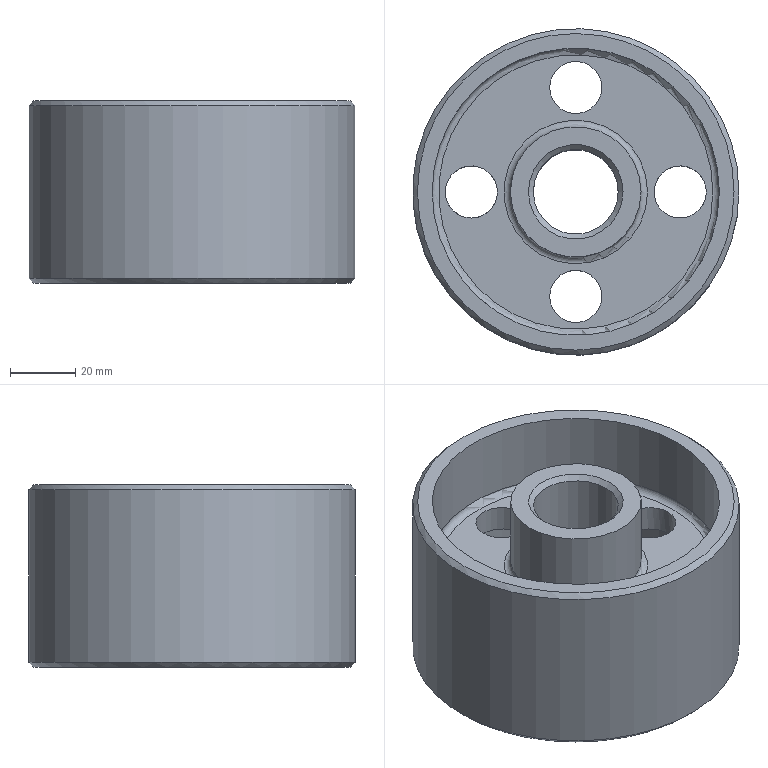Part | NX | features EXTRUDE 5, DATUM_CSYS 3, CHAMFER 2, SKETCH 2, BLEND 1 | 1 solid | 24 faces | box 100 x 100 x 56 mm | volume 171833 mm3 | cylinder 10 | plane 6 | cone 4 | torus 4 | commonest cylinder face diameters 16 x4 40 x2 88 x2 26 x1 100 x1
STEP:
#1=CARTESIAN_POINT('',(14.5,0.,56.));
#2=VERTEX_POINT('',#1);
#3=CARTESIAN_POINT('',(0.,0.,56.));
#4=DIRECTION('',(0.,0.,1.));
#5=DIRECTION('',(1.,0.,0.));
#6=AXIS2_PLACEMENT_3D('',#3,#4,#5);
#7=CIRCLE('',#6,14.5);
#8=EDGE_CURVE('',#2,#2,#7,.F.);
#9=ORIENTED_EDGE('',*,*,#8,.T.);
#10=EDGE_LOOP('',(#9));
#11=FACE_BOUND('',#10,.T.);
#12=CARTESIAN_POINT('',(20.,0.,56.));
#13=VERTEX_POINT('',#12);
#14=CARTESIAN_POINT('',(0.,0.,56.));
#15=DIRECTION('',(0.,0.,1.));
#16=DIRECTION('',(1.,0.,0.));
#17=AXIS2_PLACEMENT_3D('',#14,#15,#16);
#18=CIRCLE('',#17,20.);
#19=EDGE_CURVE('',#13,#13,#18,.T.);
#20=ORIENTED_EDGE('',*,*,#19,.T.);
#21=EDGE_LOOP('',(#20));
#22=FACE_BOUND('',#21,.T.);
#23=CARTESIAN_POINT('',(0.,0.,56.));
#24=DIRECTION('',(0.,0.,1.));
#25=DIRECTION('',(1.,0.,0.));
#26=AXIS2_PLACEMENT_3D('',#23,#24,#25);
#27=PLANE('',#26);
#28=ADVANCED_FACE('',(#11,#22),#27,.T.);
#29=CARTESIAN_POINT('',(48.5,0.,0.));
#30=VERTEX_POINT('',#29);
#31=CARTESIAN_POINT('',(0.,0.,0.));
#32=DIRECTION('',(0.,0.,1.));
#33=DIRECTION('',(1.,0.,0.));
#34=AXIS2_PLACEMENT_3D('',#31,#32,#33);
#35=CIRCLE('',#34,48.5);
#36=EDGE_CURVE('',#30,#30,#35,.F.);
#37=ORIENTED_EDGE('',*,*,#36,.T.);
#38=EDGE_LOOP('',(#37));
#39=FACE_BOUND('',#38,.T.);
#40=CARTESIAN_POINT('',(44.,0.,0.));
#41=VERTEX_POINT('',#40);
#42=CARTESIAN_POINT('',(0.,0.,0.));
#43=DIRECTION('',(0.,0.,-1.));
#44=DIRECTION('',(1.,0.,0.));
#45=AXIS2_PLACEMENT_3D('',#42,#43,#44);
#46=CIRCLE('',#45,44.);
#47=EDGE_CURVE('',#41,#41,#46,.T.);
#48=ORIENTED_EDGE('',*,*,#47,.F.);
#49=EDGE_LOOP('',(#48));
#50=FACE_BOUND('',#49,.T.);
#51=CARTESIAN_POINT('',(0.,0.,0.));
#52=DIRECTION('',(0.,0.,1.));
#53=DIRECTION('',(1.,0.,0.));
#54=AXIS2_PLACEMENT_3D('',#51,#52,#53);
#55=PLANE('',#54);
#56=ADVANCED_FACE('',(#39,#50),#55,.F.);
#57=CARTESIAN_POINT('',(14.5,0.,0.));
#58=VERTEX_POINT('',#57);
#59=CARTESIAN_POINT('',(0.,0.,0.));
#60=DIRECTION('',(0.,0.,1.));
#61=DIRECTION('',(1.,0.,0.));
#62=AXIS2_PLACEMENT_3D('',#59,#60,#61);
#63=CIRCLE('',#62,14.5);
#64=EDGE_CURVE('',#58,#58,#63,.T.);
#65=ORIENTED_EDGE('',*,*,#64,.T.);
#66=EDGE_LOOP('',(#65));
#67=FACE_BOUND('',#66,.T.);
#68=CARTESIAN_POINT('',(20.,0.,0.));
#69=VERTEX_POINT('',#68);
#70=CARTESIAN_POINT('',(0.,0.,0.));
#71=DIRECTION('',(0.,0.,1.));
#72=DIRECTION('',(1.,0.,0.));
#73=AXIS2_PLACEMENT_3D('',#70,#71,#72);
#74=CIRCLE('',#73,20.);
#75=EDGE_CURVE('',#69,#69,#74,.T.);
#76=ORIENTED_EDGE('',*,*,#75,.F.);
#77=EDGE_LOOP('',(#76));
#78=FACE_BOUND('',#77,.T.);
#79=CARTESIAN_POINT('',(0.,0.,0.));
#80=DIRECTION('',(0.,0.,1.));
#81=DIRECTION('',(1.,0.,0.));
#82=AXIS2_PLACEMENT_3D('',#79,#80,#81);
#83=PLANE('',#82);
#84=ADVANCED_FACE('',(#67,#78),#83,.F.);
#85=CARTESIAN_POINT('',(50.,0.,1.5));
#86=VERTEX_POINT('',#85);
#87=CARTESIAN_POINT('',(0.,0.,1.5));
#88=DIRECTION('',(0.,0.,1.));
#89=DIRECTION('',(1.,0.,0.));
#90=AXIS2_PLACEMENT_3D('',#87,#88,#89);
#91=CIRCLE('',#90,50.);
#92=EDGE_CURVE('',#86,#86,#91,.T.);
#93=ORIENTED_EDGE('',*,*,#92,.T.);
#94=EDGE_LOOP('',(#93));
#95=FACE_BOUND('',#94,.T.);
#96=CARTESIAN_POINT('',(50.,0.,54.5));
#97=VERTEX_POINT('',#96);
#98=CARTESIAN_POINT('',(0.,0.,54.5));
#99=DIRECTION('',(0.,0.,1.));
#100=DIRECTION('',(1.,0.,0.));
#101=AXIS2_PLACEMENT_3D('',#98,#99,#100);
#102=CIRCLE('',#101,50.);
#103=EDGE_CURVE('',#97,#97,#102,.F.);
#104=ORIENTED_EDGE('',*,*,#103,.T.);
#105=EDGE_LOOP('',(#104));
#106=FACE_BOUND('',#105,.T.);
#107=CARTESIAN_POINT('',(0.,0.,56.));
#108=DIRECTION('',(0.,0.,-1.));
#109=DIRECTION('',(-1.,0.,0.));
#110=AXIS2_PLACEMENT_3D('',#107,#108,#109);
#111=CYLINDRICAL_SURFACE('',#110,50.);
#112=ADVANCED_FACE('',(#95,#106),#111,.T.);
#113=CARTESIAN_POINT('',(48.5,0.,56.));
#114=VERTEX_POINT('',#113);
#115=CARTESIAN_POINT('',(0.,0.,56.));
#116=DIRECTION('',(0.,0.,1.));
#117=DIRECTION('',(1.,0.,0.));
#118=AXIS2_PLACEMENT_3D('',#115,#116,#117);
#119=CIRCLE('',#118,48.5);
#120=EDGE_CURVE('',#114,#114,#119,.T.);
#121=ORIENTED_EDGE('',*,*,#120,.T.);
#122=EDGE_LOOP('',(#121));
#123=FACE_BOUND('',#122,.T.);
#124=CARTESIAN_POINT('',(44.,0.,56.));
#125=VERTEX_POINT('',#124);
#126=CARTESIAN_POINT('',(0.,0.,56.));
#127=DIRECTION('',(0.,0.,1.));
#128=DIRECTION('',(1.,0.,0.));
#129=AXIS2_PLACEMENT_3D('',#126,#127,#128);
#130=CIRCLE('',#129,44.);
#131=EDGE_CURVE('',#125,#125,#130,.T.);
#132=ORIENTED_EDGE('',*,*,#131,.F.);
#133=EDGE_LOOP('',(#132));
#134=FACE_BOUND('',#133,.T.);
#135=CARTESIAN_POINT('',(0.,0.,56.));
#136=DIRECTION('',(0.,0.,1.));
#137=DIRECTION('',(1.,0.,0.));
#138=AXIS2_PLACEMENT_3D('',#135,#136,#137);
#139=PLANE('',#138);
#140=ADVANCED_FACE('',(#123,#134),#139,.T.);
#141=CARTESIAN_POINT('',(13.,0.,54.5));
#142=VERTEX_POINT('',#141);
#143=CARTESIAN_POINT('',(0.,0.,54.5));
#144=DIRECTION('',(0.,0.,1.));
#145=DIRECTION('',(1.,0.,0.));
#146=AXIS2_PLACEMENT_3D('',#143,#144,#145);
#147=CIRCLE('',#146,13.);
#148=EDGE_CURVE('',#142,#142,#147,.T.);
#149=ORIENTED_EDGE('',*,*,#148,.T.);
#150=EDGE_LOOP('',(#149));
#151=FACE_BOUND('',#150,.T.);
#152=CARTESIAN_POINT('',(13.,0.,1.5));
#153=VERTEX_POINT('',#152);
#154=CARTESIAN_POINT('',(0.,0.,1.5));
#155=DIRECTION('',(0.,0.,1.));
#156=DIRECTION('',(1.,0.,0.));
#157=AXIS2_PLACEMENT_3D('',#154,#155,#156);
#158=CIRCLE('',#157,13.);
#159=EDGE_CURVE('',#153,#153,#158,.F.);
#160=ORIENTED_EDGE('',*,*,#159,.T.);
#161=EDGE_LOOP('',(#160));
#162=FACE_BOUND('',#161,.T.);
#163=CARTESIAN_POINT('',(0.,0.,56.));
#164=DIRECTION('',(0.,0.,-1.));
#165=DIRECTION('',(-1.,0.,0.));
#166=AXIS2_PLACEMENT_3D('',#163,#164,#165);
#167=CYLINDRICAL_SURFACE('',#166,13.);
#168=ADVANCED_FACE('',(#151,#162),#167,.F.);
#169=CARTESIAN_POINT('',(-44.,0.,22.));
#170=VERTEX_POINT('',#169);
#171=CARTESIAN_POINT('',(0.,0.,22.));
#172=DIRECTION('',(0.,0.,-1.));
#173=DIRECTION('',(-1.,0.,0.));
#174=AXIS2_PLACEMENT_3D('',#171,#172,#173);
#175=CIRCLE('',#174,44.);
#176=EDGE_CURVE('',#170,#170,#175,.F.);
#177=ORIENTED_EDGE('',*,*,#176,.T.);
#178=EDGE_LOOP('',(#177));
#179=FACE_BOUND('',#178,.T.);
#180=ORIENTED_EDGE('',*,*,#47,.T.);
#181=EDGE_LOOP('',(#180));
#182=FACE_BOUND('',#181,.T.);
#183=CARTESIAN_POINT('',(0.,0.,24.));
#184=DIRECTION('',(0.,0.,-1.));
#185=DIRECTION('',(-1.,0.,0.));
#186=AXIS2_PLACEMENT_3D('',#183,#184,#185);
#187=CYLINDRICAL_SURFACE('',#186,44.);
#188=ADVANCED_FACE('',(#179,#182),#187,.F.);
#189=CARTESIAN_POINT('',(-20.,0.,22.));
#190=VERTEX_POINT('',#189);
#191=CARTESIAN_POINT('',(0.,0.,22.));
#192=DIRECTION('',(0.,0.,-1.));
#193=DIRECTION('',(-1.,0.,0.));
#194=AXIS2_PLACEMENT_3D('',#191,#192,#193);
#195=CIRCLE('',#194,20.);
#196=EDGE_CURVE('',#190,#190,#195,.T.);
#197=ORIENTED_EDGE('',*,*,#196,.T.);
#198=EDGE_LOOP('',(#197));
#199=FACE_BOUND('',#198,.T.);
#200=ORIENTED_EDGE('',*,*,#75,.T.);
#201=EDGE_LOOP('',(#200));
#202=FACE_BOUND('',#201,.T.);
#203=CARTESIAN_POINT('',(0.,0.,24.));
#204=DIRECTION('',(0.,0.,-1.));
#205=DIRECTION('',(-1.,0.,0.));
#206=AXIS2_PLACEMENT_3D('',#203,#204,#205);
#207=CYLINDRICAL_SURFACE('',#206,20.);
#208=ADVANCED_FACE('',(#199,#202),#207,.T.);
#209=CARTESIAN_POINT('',(-22.,0.,24.));
#210=VERTEX_POINT('',#209);
#211=CARTESIAN_POINT('',(0.,0.,24.));
#212=DIRECTION('',(0.,0.,-1.));
#213=DIRECTION('',(-1.,0.,0.));
#214=AXIS2_PLACEMENT_3D('',#211,#212,#213);
#215=CIRCLE('',#214,22.);
#216=EDGE_CURVE('',#210,#210,#215,.F.);
#217=ORIENTED_EDGE('',*,*,#216,.T.);
#218=EDGE_LOOP('',(#217));
#219=FACE_BOUND('',#218,.T.);
#220=CARTESIAN_POINT('',(-42.,0.,24.));
#221=VERTEX_POINT('',#220);
#222=CARTESIAN_POINT('',(0.,0.,24.));
#223=DIRECTION('',(0.,0.,-1.));
#224=DIRECTION('',(-1.,0.,0.));
#225=AXIS2_PLACEMENT_3D('',#222,#223,#224);
#226=CIRCLE('',#225,42.);
#227=EDGE_CURVE('',#221,#221,#226,.T.);
#228=ORIENTED_EDGE('',*,*,#227,.T.);
#229=EDGE_LOOP('',(#228));
#230=FACE_BOUND('',#229,.T.);
#231=CARTESIAN_POINT('',(-8.,32.,24.));
#232=VERTEX_POINT('',#231);
#233=CARTESIAN_POINT('',(0.,32.,24.));
#234=DIRECTION('',(0.,0.,-1.));
#235=DIRECTION('',(-1.,0.,0.));
#236=AXIS2_PLACEMENT_3D('',#233,#234,#235);
#237=CIRCLE('',#236,8.);
#238=EDGE_CURVE('',#232,#232,#237,.T.);
#239=ORIENTED_EDGE('',*,*,#238,.F.);
#240=EDGE_LOOP('',(#239));
#241=FACE_BOUND('',#240,.T.);
#242=CARTESIAN_POINT('',(-32.,-8.,24.));
#243=VERTEX_POINT('',#242);
#244=CARTESIAN_POINT('',(-32.,0.,24.));
#245=DIRECTION('',(0.,0.,-1.));
#246=DIRECTION('',(0.,-1.,0.));
#247=AXIS2_PLACEMENT_3D('',#244,#245,#246);
#248=CIRCLE('',#247,8.);
#249=EDGE_CURVE('',#243,#243,#248,.T.);
#250=ORIENTED_EDGE('',*,*,#249,.F.);
#251=EDGE_LOOP('',(#250));
#252=FACE_BOUND('',#251,.T.);
#253=CARTESIAN_POINT('',(8.,-32.,24.));
#254=VERTEX_POINT('',#253);
#255=CARTESIAN_POINT('',(0.,-32.,24.));
#256=DIRECTION('',(0.,0.,-1.));
#257=DIRECTION('',(1.,0.,0.));
#258=AXIS2_PLACEMENT_3D('',#255,#256,#257);
#259=CIRCLE('',#258,8.);
#260=EDGE_CURVE('',#254,#254,#259,.T.);
#261=ORIENTED_EDGE('',*,*,#260,.F.);
#262=EDGE_LOOP('',(#261));
#263=FACE_BOUND('',#262,.T.);
#264=CARTESIAN_POINT('',(32.,8.,24.));
#265=VERTEX_POINT('',#264);
#266=CARTESIAN_POINT('',(32.,0.,24.));
#267=DIRECTION('',(0.,0.,-1.));
#268=DIRECTION('',(0.,1.,0.));
#269=AXIS2_PLACEMENT_3D('',#266,#267,#268);
#270=CIRCLE('',#269,8.);
#271=EDGE_CURVE('',#265,#265,#270,.T.);
#272=ORIENTED_EDGE('',*,*,#271,.F.);
#273=EDGE_LOOP('',(#272));
#274=FACE_BOUND('',#273,.T.);
#275=CARTESIAN_POINT('',(0.,0.,24.));
#276=DIRECTION('',(0.,0.,-1.));
#277=DIRECTION('',(-1.,0.,0.));
#278=AXIS2_PLACEMENT_3D('',#275,#276,#277);
#279=PLANE('',#278);
#280=ADVANCED_FACE('',(#219,#230,#241,#252,#263,#274),#279,.T.);
#281=CARTESIAN_POINT('',(44.,0.,34.));
#282=VERTEX_POINT('',#281);
#283=CARTESIAN_POINT('',(0.,0.,34.));
#284=DIRECTION('',(0.,0.,1.));
#285=DIRECTION('',(1.,0.,0.));
#286=AXIS2_PLACEMENT_3D('',#283,#284,#285);
#287=CIRCLE('',#286,44.);
#288=EDGE_CURVE('',#282,#282,#287,.F.);
#289=ORIENTED_EDGE('',*,*,#288,.T.);
#290=EDGE_LOOP('',(#289));
#291=FACE_BOUND('',#290,.T.);
#292=ORIENTED_EDGE('',*,*,#131,.T.);
#293=EDGE_LOOP('',(#292));
#294=FACE_BOUND('',#293,.T.);
#295=CARTESIAN_POINT('',(0.,0.,56.));
#296=DIRECTION('',(0.,0.,-1.));
#297=DIRECTION('',(-1.,0.,0.));
#298=AXIS2_PLACEMENT_3D('',#295,#296,#297);
#299=CYLINDRICAL_SURFACE('',#298,44.);
#300=ADVANCED_FACE('',(#291,#294),#299,.F.);
#301=CARTESIAN_POINT('',(20.,0.,34.));
#302=VERTEX_POINT('',#301);
#303=CARTESIAN_POINT('',(0.,0.,34.));
#304=DIRECTION('',(0.,0.,1.));
#305=DIRECTION('',(1.,0.,0.));
#306=AXIS2_PLACEMENT_3D('',#303,#304,#305);
#307=CIRCLE('',#306,20.);
#308=EDGE_CURVE('',#302,#302,#307,.T.);
#309=ORIENTED_EDGE('',*,*,#308,.T.);
#310=EDGE_LOOP('',(#309));
#311=FACE_BOUND('',#310,.T.);
#312=ORIENTED_EDGE('',*,*,#19,.F.);
#313=EDGE_LOOP('',(#312));
#314=FACE_BOUND('',#313,.T.);
#315=CARTESIAN_POINT('',(0.,0.,56.));
#316=DIRECTION('',(0.,0.,-1.));
#317=DIRECTION('',(-1.,0.,0.));
#318=AXIS2_PLACEMENT_3D('',#315,#316,#317);
#319=CYLINDRICAL_SURFACE('',#318,20.);
#320=ADVANCED_FACE('',(#311,#314),#319,.T.);
#321=CARTESIAN_POINT('',(22.,0.,32.));
#322=VERTEX_POINT('',#321);
#323=CARTESIAN_POINT('',(0.,0.,32.));
#324=DIRECTION('',(0.,0.,1.));
#325=DIRECTION('',(1.,0.,0.));
#326=AXIS2_PLACEMENT_3D('',#323,#324,#325);
#327=CIRCLE('',#326,22.);
#328=EDGE_CURVE('',#322,#322,#327,.F.);
#329=ORIENTED_EDGE('',*,*,#328,.T.);
#330=EDGE_LOOP('',(#329));
#331=FACE_BOUND('',#330,.T.);
#332=CARTESIAN_POINT('',(42.,0.,32.));
#333=VERTEX_POINT('',#332);
#334=CARTESIAN_POINT('',(0.,0.,32.));
#335=DIRECTION('',(0.,0.,1.));
#336=DIRECTION('',(1.,0.,0.));
#337=AXIS2_PLACEMENT_3D('',#334,#335,#336);
#338=CIRCLE('',#337,42.);
#339=EDGE_CURVE('',#333,#333,#338,.T.);
#340=ORIENTED_EDGE('',*,*,#339,.T.);
#341=EDGE_LOOP('',(#340));
#342=FACE_BOUND('',#341,.T.);
#343=CARTESIAN_POINT('',(8.,32.,32.));
#344=VERTEX_POINT('',#343);
#345=CARTESIAN_POINT('',(0.,32.,32.));
#346=DIRECTION('',(0.,0.,1.));
#347=DIRECTION('',(1.,0.,0.));
#348=AXIS2_PLACEMENT_3D('',#345,#346,#347);
#349=CIRCLE('',#348,8.);
#350=EDGE_CURVE('',#344,#344,#349,.T.);
#351=ORIENTED_EDGE('',*,*,#350,.F.);
#352=EDGE_LOOP('',(#351));
#353=FACE_BOUND('',#352,.T.);
#354=CARTESIAN_POINT('',(-24.,0.,32.));
#355=VERTEX_POINT('',#354);
#356=CARTESIAN_POINT('',(-32.,0.,32.));
#357=DIRECTION('',(0.,0.,1.));
#358=DIRECTION('',(1.,0.,0.));
#359=AXIS2_PLACEMENT_3D('',#356,#357,#358);
#360=CIRCLE('',#359,8.);
#361=EDGE_CURVE('',#355,#355,#360,.T.);
#362=ORIENTED_EDGE('',*,*,#361,.F.);
#363=EDGE_LOOP('',(#362));
#364=FACE_BOUND('',#363,.T.);
#365=CARTESIAN_POINT('',(8.,-32.,32.));
#366=VERTEX_POINT('',#365);
#367=CARTESIAN_POINT('',(0.,-32.,32.));
#368=DIRECTION('',(0.,0.,1.));
#369=DIRECTION('',(1.,0.,0.));
#370=AXIS2_PLACEMENT_3D('',#367,#368,#369);
#371=CIRCLE('',#370,8.);
#372=EDGE_CURVE('',#366,#366,#371,.T.);
#373=ORIENTED_EDGE('',*,*,#372,.F.);
#374=EDGE_LOOP('',(#373));
#375=FACE_BOUND('',#374,.T.);
#376=CARTESIAN_POINT('',(40.,0.,32.));
#377=VERTEX_POINT('',#376);
#378=CARTESIAN_POINT('',(32.,0.,32.));
#379=DIRECTION('',(0.,0.,1.));
#380=DIRECTION('',(1.,0.,0.));
#381=AXIS2_PLACEMENT_3D('',#378,#379,#380);
#382=CIRCLE('',#381,8.);
#383=EDGE_CURVE('',#377,#377,#382,.T.);
#384=ORIENTED_EDGE('',*,*,#383,.F.);
#385=EDGE_LOOP('',(#384));
#386=FACE_BOUND('',#385,.T.);
#387=CARTESIAN_POINT('',(0.,0.,32.));
#388=DIRECTION('',(0.,0.,1.));
#389=DIRECTION('',(1.,0.,0.));
#390=AXIS2_PLACEMENT_3D('',#387,#388,#389);
#391=PLANE('',#390);
#392=ADVANCED_FACE('',(#331,#342,#353,#364,#375,#386),#391,.T.);
#393=ORIENTED_EDGE('',*,*,#383,.T.);
#394=EDGE_LOOP('',(#393));
#395=FACE_BOUND('',#394,.T.);
#396=ORIENTED_EDGE('',*,*,#271,.T.);
#397=EDGE_LOOP('',(#396));
#398=FACE_BOUND('',#397,.T.);
#399=CARTESIAN_POINT('',(32.,0.,80.));
#400=DIRECTION('',(0.,0.,-1.));
#401=DIRECTION('',(-1.,0.,0.));
#402=AXIS2_PLACEMENT_3D('',#399,#400,#401);
#403=CYLINDRICAL_SURFACE('',#402,8.);
#404=ADVANCED_FACE('',(#395,#398),#403,.F.);
#405=ORIENTED_EDGE('',*,*,#372,.T.);
#406=EDGE_LOOP('',(#405));
#407=FACE_BOUND('',#406,.T.);
#408=ORIENTED_EDGE('',*,*,#260,.T.);
#409=EDGE_LOOP('',(#408));
#410=FACE_BOUND('',#409,.T.);
#411=CARTESIAN_POINT('',(0.,-32.,80.));
#412=DIRECTION('',(0.,0.,-1.));
#413=DIRECTION('',(-1.,0.,0.));
#414=AXIS2_PLACEMENT_3D('',#411,#412,#413);
#415=CYLINDRICAL_SURFACE('',#414,8.);
#416=ADVANCED_FACE('',(#407,#410),#415,.F.);
#417=ORIENTED_EDGE('',*,*,#361,.T.);
#418=EDGE_LOOP('',(#417));
#419=FACE_BOUND('',#418,.T.);
#420=ORIENTED_EDGE('',*,*,#249,.T.);
#421=EDGE_LOOP('',(#420));
#422=FACE_BOUND('',#421,.T.);
#423=CARTESIAN_POINT('',(-32.,0.,80.));
#424=DIRECTION('',(0.,0.,-1.));
#425=DIRECTION('',(-1.,0.,0.));
#426=AXIS2_PLACEMENT_3D('',#423,#424,#425);
#427=CYLINDRICAL_SURFACE('',#426,8.);
#428=ADVANCED_FACE('',(#419,#422),#427,.F.);
#429=ORIENTED_EDGE('',*,*,#350,.T.);
#430=EDGE_LOOP('',(#429));
#431=FACE_BOUND('',#430,.T.);
#432=ORIENTED_EDGE('',*,*,#238,.T.);
#433=EDGE_LOOP('',(#432));
#434=FACE_BOUND('',#433,.T.);
#435=CARTESIAN_POINT('',(0.,32.,80.));
#436=DIRECTION('',(0.,0.,-1.));
#437=DIRECTION('',(-1.,0.,0.));
#438=AXIS2_PLACEMENT_3D('',#435,#436,#437);
#439=CYLINDRICAL_SURFACE('',#438,8.);
#440=ADVANCED_FACE('',(#431,#434),#439,.F.);
#441=ORIENTED_EDGE('',*,*,#36,.F.);
#442=EDGE_LOOP('',(#441));
#443=FACE_BOUND('',#442,.T.);
#444=ORIENTED_EDGE('',*,*,#92,.F.);
#445=EDGE_LOOP('',(#444));
#446=FACE_BOUND('',#445,.T.);
#447=CARTESIAN_POINT('',(0.,0.,1.5));
#448=DIRECTION('',(0.,0.,1.));
#449=DIRECTION('',(1.,0.,0.));
#450=AXIS2_PLACEMENT_3D('',#447,#448,#449);
#451=CONICAL_SURFACE('',#450,50.,0.7854);
#452=ADVANCED_FACE('',(#443,#446),#451,.T.);
#453=ORIENTED_EDGE('',*,*,#103,.F.);
#454=EDGE_LOOP('',(#453));
#455=FACE_BOUND('',#454,.T.);
#456=ORIENTED_EDGE('',*,*,#120,.F.);
#457=EDGE_LOOP('',(#456));
#458=FACE_BOUND('',#457,.T.);
#459=CARTESIAN_POINT('',(0.,0.,56.));
#460=DIRECTION('',(0.,0.,-1.));
#461=DIRECTION('',(-1.,0.,0.));
#462=AXIS2_PLACEMENT_3D('',#459,#460,#461);
#463=CONICAL_SURFACE('',#462,48.5,0.7854);
#464=ADVANCED_FACE('',(#455,#458),#463,.T.);
#465=ORIENTED_EDGE('',*,*,#148,.F.);
#466=EDGE_LOOP('',(#465));
#467=FACE_BOUND('',#466,.T.);
#468=ORIENTED_EDGE('',*,*,#8,.F.);
#469=EDGE_LOOP('',(#468));
#470=FACE_BOUND('',#469,.T.);
#471=CARTESIAN_POINT('',(0.,0.,56.));
#472=DIRECTION('',(0.,0.,1.));
#473=DIRECTION('',(1.,0.,0.));
#474=AXIS2_PLACEMENT_3D('',#471,#472,#473);
#475=CONICAL_SURFACE('',#474,14.5,0.7854);
#476=ADVANCED_FACE('',(#467,#470),#475,.F.);
#477=ORIENTED_EDGE('',*,*,#64,.F.);
#478=EDGE_LOOP('',(#477));
#479=FACE_BOUND('',#478,.T.);
#480=ORIENTED_EDGE('',*,*,#159,.F.);
#481=EDGE_LOOP('',(#480));
#482=FACE_BOUND('',#481,.T.);
#483=CARTESIAN_POINT('',(0.,0.,1.5));
#484=DIRECTION('',(0.,0.,-1.));
#485=DIRECTION('',(-1.,0.,0.));
#486=AXIS2_PLACEMENT_3D('',#483,#484,#485);
#487=CONICAL_SURFACE('',#486,13.,0.7854);
#488=ADVANCED_FACE('',(#479,#482),#487,.F.);
#489=ORIENTED_EDGE('',*,*,#216,.F.);
#490=EDGE_LOOP('',(#489));
#491=FACE_BOUND('',#490,.T.);
#492=ORIENTED_EDGE('',*,*,#196,.F.);
#493=EDGE_LOOP('',(#492));
#494=FACE_BOUND('',#493,.T.);
#495=CARTESIAN_POINT('',(0.,0.,22.));
#496=DIRECTION('',(0.,0.,-1.));
#497=DIRECTION('',(-1.,0.,0.));
#498=AXIS2_PLACEMENT_3D('',#495,#496,#497);
#499=TOROIDAL_SURFACE('',#498,22.,2.);
#500=ADVANCED_FACE('',(#491,#494),#499,.F.);
#501=ORIENTED_EDGE('',*,*,#227,.F.);
#502=EDGE_LOOP('',(#501));
#503=FACE_BOUND('',#502,.T.);
#504=ORIENTED_EDGE('',*,*,#176,.F.);
#505=EDGE_LOOP('',(#504));
#506=FACE_BOUND('',#505,.T.);
#507=CARTESIAN_POINT('',(0.,0.,22.));
#508=DIRECTION('',(0.,0.,-1.));
#509=DIRECTION('',(-1.,0.,0.));
#510=AXIS2_PLACEMENT_3D('',#507,#508,#509);
#511=TOROIDAL_SURFACE('',#510,42.,2.);
#512=ADVANCED_FACE('',(#503,#506),#511,.F.);
#513=ORIENTED_EDGE('',*,*,#308,.F.);
#514=EDGE_LOOP('',(#513));
#515=FACE_BOUND('',#514,.T.);
#516=ORIENTED_EDGE('',*,*,#328,.F.);
#517=EDGE_LOOP('',(#516));
#518=FACE_BOUND('',#517,.T.);
#519=CARTESIAN_POINT('',(0.,0.,34.));
#520=DIRECTION('',(0.,0.,1.));
#521=DIRECTION('',(1.,0.,0.));
#522=AXIS2_PLACEMENT_3D('',#519,#520,#521);
#523=TOROIDAL_SURFACE('',#522,22.,2.);
#524=ADVANCED_FACE('',(#515,#518),#523,.F.);
#525=ORIENTED_EDGE('',*,*,#339,.F.);
#526=EDGE_LOOP('',(#525));
#527=FACE_BOUND('',#526,.T.);
#528=ORIENTED_EDGE('',*,*,#288,.F.);
#529=EDGE_LOOP('',(#528));
#530=FACE_BOUND('',#529,.T.);
#531=CARTESIAN_POINT('',(0.,0.,34.));
#532=DIRECTION('',(0.,0.,1.));
#533=DIRECTION('',(1.,0.,0.));
#534=AXIS2_PLACEMENT_3D('',#531,#532,#533);
#535=TOROIDAL_SURFACE('',#534,42.,2.);
#536=ADVANCED_FACE('',(#527,#530),#535,.F.);
#537=CLOSED_SHELL('',(#28,#56,#84,#112,#140,#168,#188,#208,#280,#300,#320,#392,#404,#416,#428,#440,#452,#464,#476,#488,#500,#512,#524,#536));
#538=MANIFOLD_SOLID_BREP('',#537);
#539=(LENGTH_UNIT()NAMED_UNIT(*)SI_UNIT(.MILLI.,.METRE.));
#540=UNCERTAINTY_MEASURE_WITH_UNIT(LENGTH_MEASURE(0.00001),#539,'','');
#541=(NAMED_UNIT(*)PLANE_ANGLE_UNIT()SI_UNIT($,.RADIAN.));
#542=(NAMED_UNIT(*)SI_UNIT($,.STERADIAN.)SOLID_ANGLE_UNIT());
#543=(GEOMETRIC_REPRESENTATION_CONTEXT(3)GLOBAL_UNCERTAINTY_ASSIGNED_CONTEXT((#540))GLOBAL_UNIT_ASSIGNED_CONTEXT((#539,#541,#542))REPRESENTATION_CONTEXT('',''));
#544=ADVANCED_BREP_SHAPE_REPRESENTATION('',(#538),#543);